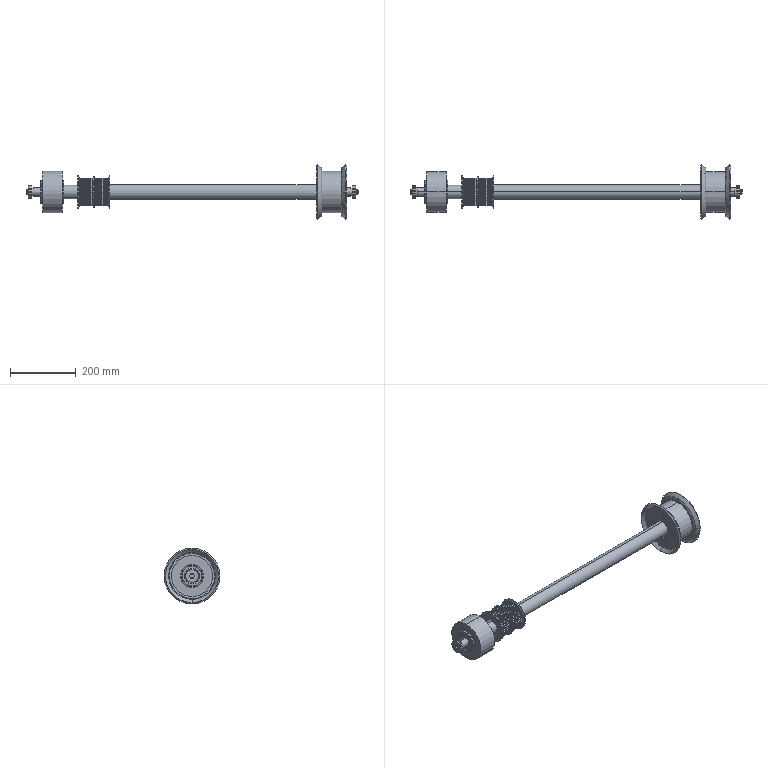Part | SolidWorks | 33 solids | 1758 faces | box 1011 x 169.042 x 169.042 mm | volume 2962647 mm3 | cylinder 820 | plane 494 | cone 272 | spline 172 | commonest cylinder face diameters 6 x200 1.6 x168 5.14 x168 85.208 x70 5 x16 6.6 x16